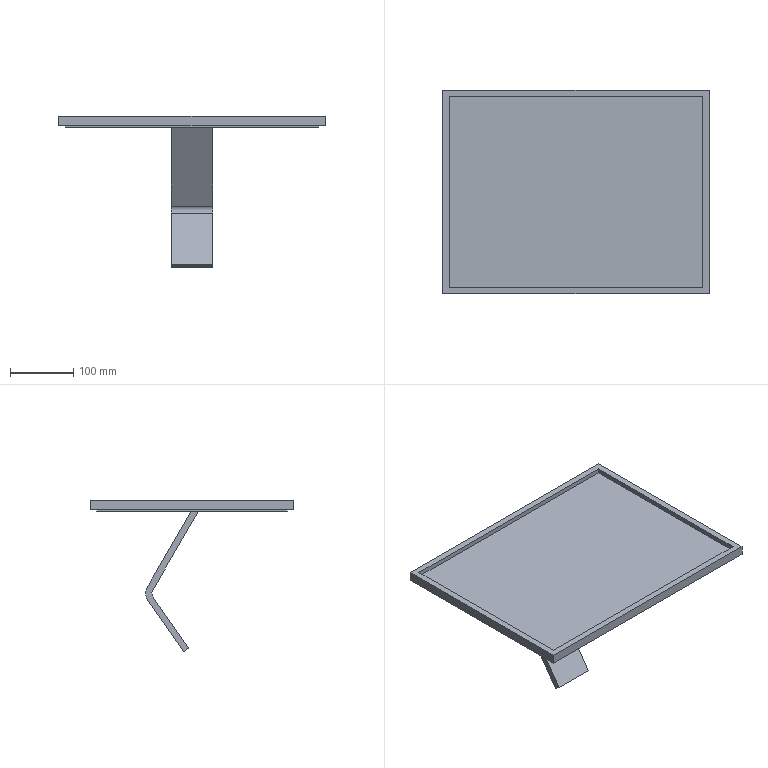Part | STEP file | Computer | 1 solid | 25 faces | box 420 x 320 x 238.828 mm | volume 1582397 mm3 | plane 23 | cylinder 2 | commonest cylinder face diameters 20 x1 40 x1